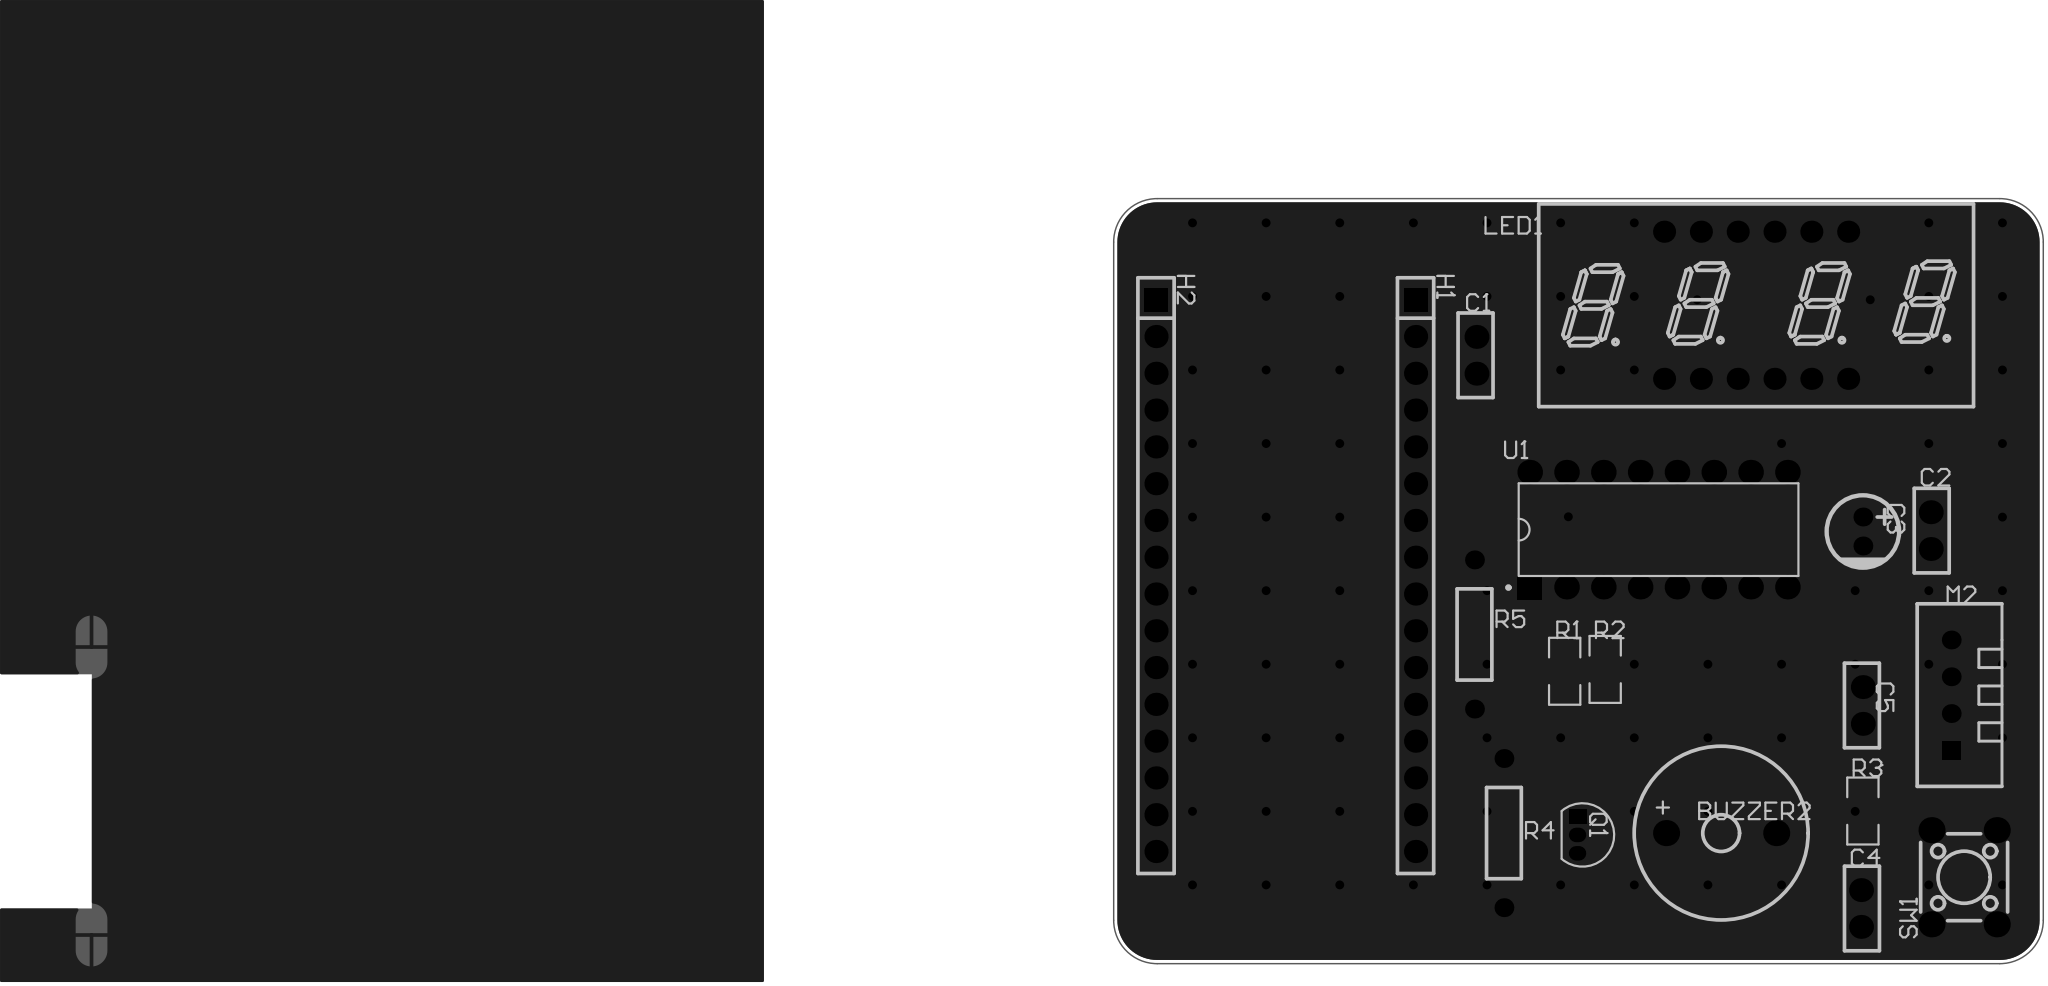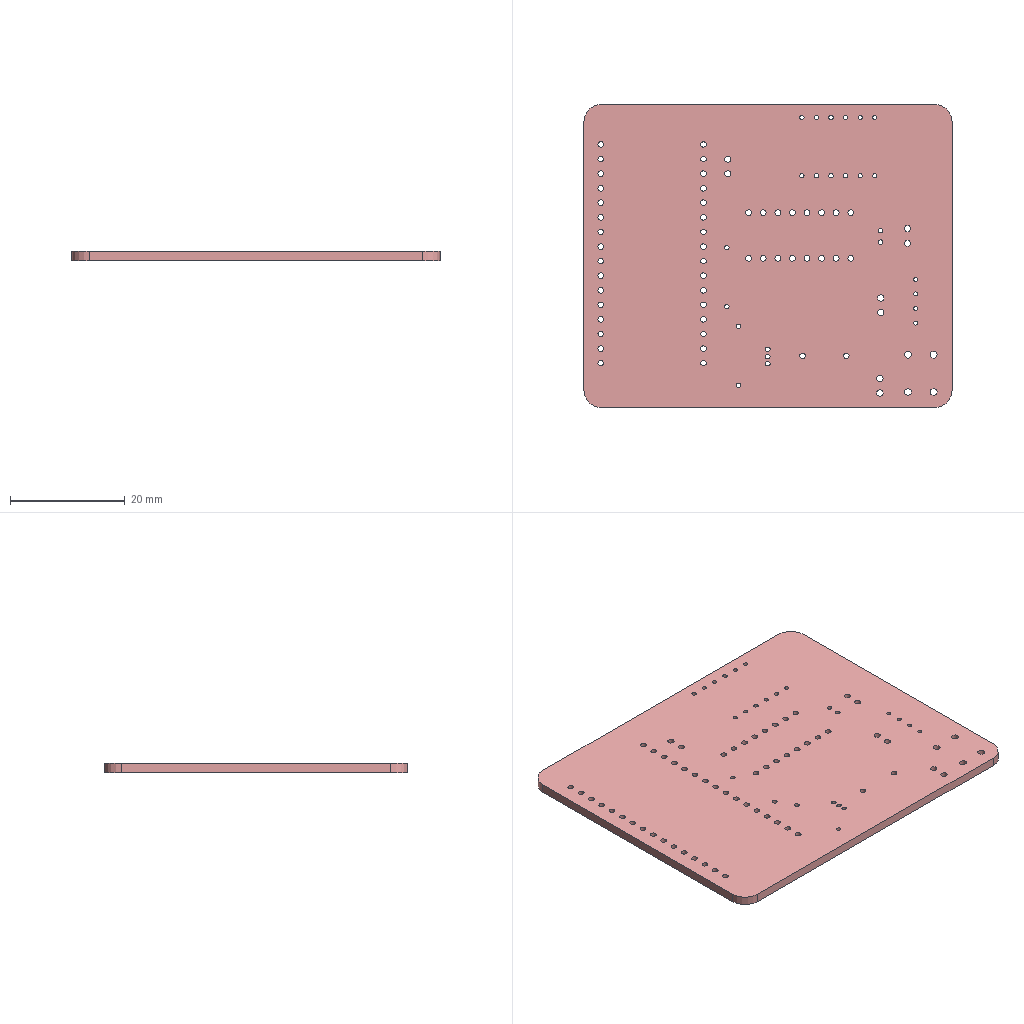Circuit board layout | Altium Designer | box 64.1 x 52.8 x 1.6 mm
Layer stack:
# Altium Designer layer stack of  (unit mm; dielectric type: 0 none, 1 core, 2 prepreg, 3 surface material)
index,name,kind,layer,copper_thickness_mm,dielectric_type,dielectric_thickness_mm,dielectric_material,dielectric_constant
0,Top Paste Mask Layer,other,,,,,,
1,Top Silkscreen Layer,other,,,,,,
2,Top Solder Mask Layer,dielectric,,,3,0.01,,3.3
3,Top Layer,copper,Top Layer,0.035,,,,
4,Dielectric1,dielectric,,,3,1.51,FR4,4.5
5,Bottom Layer,copper,Bottom Layer,0.035,,,,
6,Bottom Solder Mask Layer,dielectric,,,3,0.01,,3.3
7,Bottom Silkscreen Layer,other,,,,,,
8,Bottom Paste Mask Layer,other,,,,,,
# drill layer pairs: low layer,high layer
drill_pair,Top Layer,Bottom Layer
Part placement:
Designator,Comment,Layer,Footprint,Center-X(mm),Center-Y(mm),Rotation
LED1,FJ3461AH,TopLayer,LED-SEG-TH_12P-L30.0-W14.0-P2.54-S10.16-BL,207.772,147.193,0
M2,DHT11,TopLayer,SENSOR-TH_DHT11,221.234,120.269,90
U1,TM1650-DIP16,TopLayer,DIP-16_L19.3-W6.4-P2.54-LS8.0-BL,201.041,131.699,0
BUZZER2,2.3kHz,TopLayer,BUZ-TH_BD12.0-P7.60-D0.6-FD,205.359,110.744,0
C5,100nF,TopLayer,CAP-TH_L5.8-W2.4-P2.54-D0.6,215.134,119.557,270
C4,100nF,TopLayer,CAP-TH_L5.8-W2.4-P2.54-D0.6,215.011,105.537,90
R5,4.7kΩ,TopLayer,RES-TH_BD2.4-L6.3-P10.30-D0.6,188.341,124.46,270
R2,10kΩ,TopLayer,R1206,197.358,122.047,270
R4,2kΩ,TopLayer,RES-TH_BD2.4-L6.3-P10.30-D0.6,190.373,110.744,270
C3,10uF,TopLayer,CAP-TH_BD5.0-P2.00-D0.8-FD,215.138,131.572,270
C1,100nF,TopLayer,CAP-TH_L5.8-W2.4-P2.54-D0.6,188.478,143.74,270
C2,100nF,TopLayer,CAP-TH_L5.8-W2.4-P2.54-D0.6,219.822,131.632,90
R3,10kΩ,TopLayer,R1206,215.138,112.268,90
Q1,S8550,TopLayer,TO-92-3_L4.5-W3.5-P1.27-L,195.453,110.617,270
R1,10kΩ,TopLayer,R1206,194.564,121.92,270
SW1,TS665CJ,TopLayer,SW-TH_4P-L6.0-W6.0-P4.50-LS6.5,222.123,107.696,90
H1,,TopLayer,HDR-TH_16P-P2.54-V-F,184.277,128.524,270
H2,,TopLayer,HDR-TH_16P-P2.54-V-F,166.37,128.524,270
Pad and via stacks:
# Altium Designer via and pad stacks of  (unit mm). Each distinct definition once, with the count of objects using it.
# via: kind,start_layer,end_layer,hole_mm,diameter_mm,mode(0 simple;1 top-mid-bottom;2 full stack),diameter_per_layer,count,example_net
# pad: kind,layer,hole_mm,hole_type(0 round;1 square;2 slot),plating,top_size,top_shape(1 round;2 rect;3 octagon;9 rounded rect),mid_size,bottom_size,mode,footprint,size_per_layer,count,example
pad,Multi-Layer,0.762,0,plated,1.524x1.524,1,1.524x1.524,1.524x1.524,0,LED-SEG-TH_12P-L30.0-W14.0-P2.54-S10.16-BL,,12,LED1.12
pad,Multi-Layer,0.7112,0,plated,1.295x1.295,2,1.295x1.295,1.295x1.295,0,SENSOR-TH_DHT11,,1,M2.1
pad,Multi-Layer,0.7112,0,plated,1.295x1.295,1,1.295x1.295,1.295x1.295,0,SENSOR-TH_DHT11,,3,M2.2
pad,Multi-Layer,1,0,plated,1.7x1.7,2,1.7x1.7,1.7x1.7,0,DIP-16_L19.3-W6.4-P2.54-LS8.0-BL,,1,U1.1
pad,Multi-Layer,1,0,plated,1.7x1.7,1,1.7x1.7,1.7x1.7,0,DIP-16_L19.3-W6.4-P2.54-LS8.0-BL,,15,U1.2
pad,Multi-Layer,1,0,plated,1.8x1.8,1,1.8x1.8,1.8x1.8,0,BUZ-TH_BD12.0-P7.60-D0.6-FD,,2,BUZZER2.2
pad,Multi-Layer,1.1,0,plated,1.65x1.65,1,1.65x1.65,1.65x1.65,0,CAP-TH_L5.8-W2.4-P2.54-D0.6,,8,C5.1
pad,Multi-Layer,0.8,0,plated,1.3x1.3,1,1.3x1.3,1.3x1.3,0,RES-TH_BD2.4-L6.3-P10.30-D0.6,,4,R5.1
pad,Multi-Layer,0.8,0,plated,1.3x1.3,1,1.3x1.3,1.3x1.3,0,CAP-TH_BD5.0-P2.00-D0.8-FD,,2,C3.1
pad,Multi-Layer,0.7,2,plated,1x1.2,2,1x1.2,1x1.2,0,TO-92-3_L4.5-W3.5-P1.27-L,,1,Q1.1
pad,Multi-Layer,0.7,2,plated,1x1.2,1,1x1.2,1x1.2,0,TO-92-3_L4.5-W3.5-P1.27-L,,2,Q1.2
pad,Multi-Layer,1.2,0,plated,1.8x1.8,1,1.8x1.8,1.8x1.8,0,SW-TH_4P-L6.0-W6.0-P4.50-LS6.5,,4,SW1.1
pad,Multi-Layer,1,0,plated,1.6x1.6,2,1.6x1.6,1.6x1.6,0,HDR-TH_16P-P2.54-V-F,,2,H1.1
pad,Multi-Layer,1,0,plated,1.6x1.6,1,1.6x1.6,1.6x1.6,0,HDR-TH_16P-P2.54-V-F,,30,H1.2
pad,Top Layer,0,0,plated,1.208x1.701,2,1.208x1.701,1.208x1.701,0,R1206,,6,R2.2
via,Top Layer,Bottom Layer,0.3048,0.61,0,,81,VDD_3V3
Copper pours:
name,layer,net,type(0 solid;1 hatched;2 none)
Top Layer-GND,Top Layer,GND,0
Top Layer-GND 1,Top Layer,GND,0
Bottom Layer-GND,Bottom Layer,GND,0
Bottom Layer-GND 1,Bottom Layer,GND,0
Design rules, without the lines most boards share:
# Altium Designer design rules of  (exported by Altium Designer, unit mm)
# columns: name | kind | enabled | priority | scope1 | scope2 | descriptor | typed fields (field=value)
creepage | 65 | enabled | 1 | All | All | Creepage Distance Constraint =(0mil) (All),(All) |
copperRegion | 20 | enabled | 1 | (InNet('GND')) | All | Polygon Connect Rule(Relief Connect )(Conductor Width=10mil) (Relief Angle=90 Angle) (Entries=4) (Air Gap Width=10mil) ((InNet('GND'))),(All) | connect_style(0=relief,1=direct,2=none)=0 relief_conductor_width=0.254 relief_entries=4